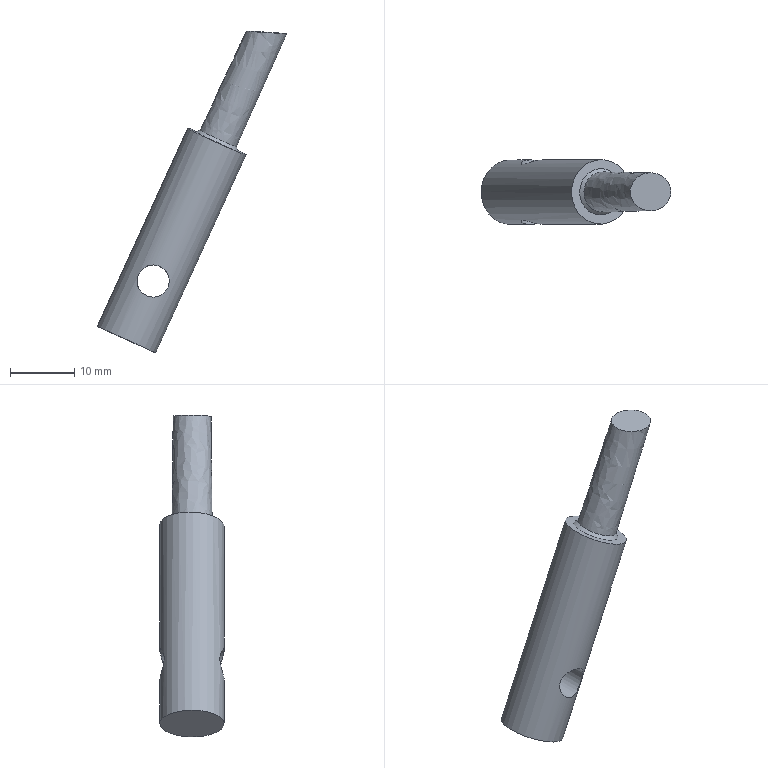Part | STEP file | solid 95 | 1 solid | 7 faces | box 29.477 x 10 x 49.99 mm | volume 3007 mm3 | cylinder 2 | plane 2 | spline 2 | cone 1 | commonest cylinder face diameters 5 x1 10 x1